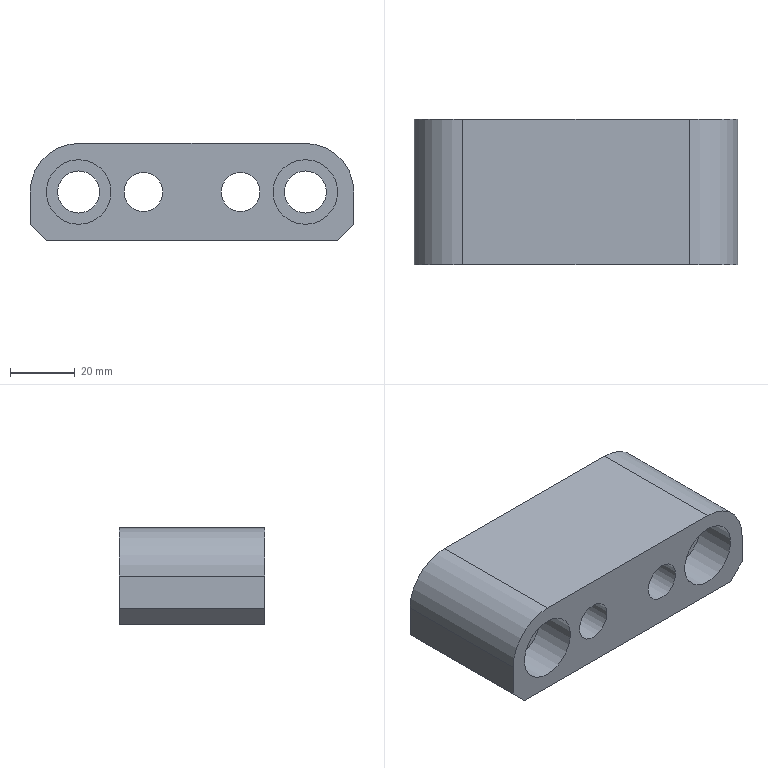Part | STEP file | solid 169 | 1 solid | 18 faces | box 100 x 45 x 30 mm | volume 102688 mm3 | plane 10 | cylinder 8 | commonest cylinder face diameters 12 x2 13 x2 20 x2 30 x2